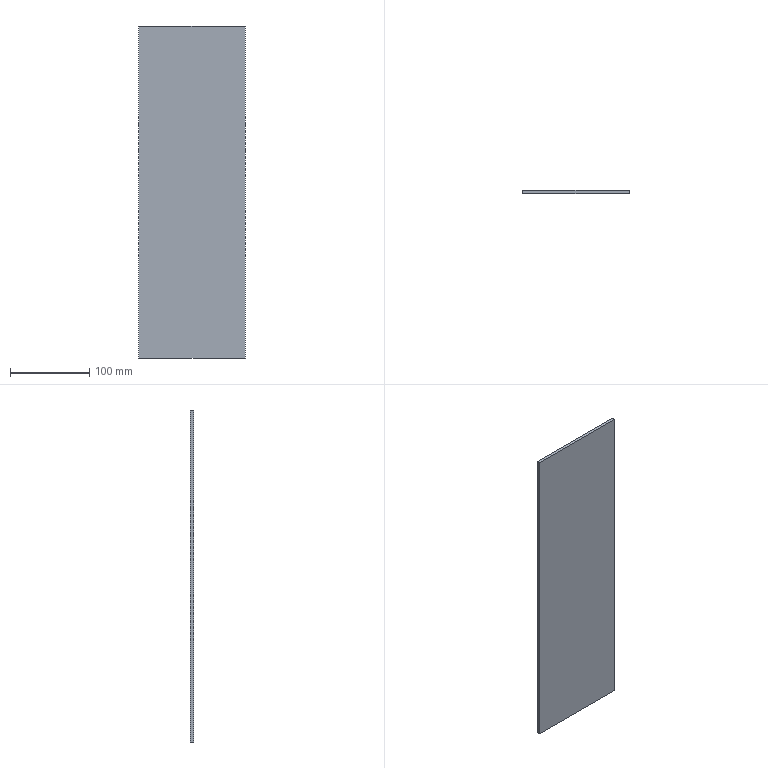Part | SolidWorks | features Extrusion 1, ICE 1 | 1 solid | 6 faces | box 135 x 4 x 420 mm | volume 226800 mm3 | plane 6
STEP:
#1=CARTESIAN_POINT('',(67.5,0.,210.));
#2=VERTEX_POINT('',#1);
#3=CARTESIAN_POINT('',(67.5,0.,-210.));
#4=VERTEX_POINT('',#3);
#5=CARTESIAN_POINT('',(67.5,0.,-210.));
#6=DIRECTION('',(0.,0.,-1.));
#7=VECTOR('',#6,1000.);
#8=LINE('',#5,#7);
#9=EDGE_CURVE('',#2,#4,#8,.T.);
#10=ORIENTED_EDGE('',*,*,#9,.T.);
#11=CARTESIAN_POINT('',(67.5,4.,-210.));
#12=VERTEX_POINT('',#11);
#13=CARTESIAN_POINT('',(67.5,4.,-210.));
#14=DIRECTION('',(0.,-1.,0.));
#15=VECTOR('',#14,1000.);
#16=LINE('',#13,#15);
#17=EDGE_CURVE('',#12,#4,#16,.T.);
#18=ORIENTED_EDGE('',*,*,#17,.F.);
#19=CARTESIAN_POINT('',(67.5,4.,210.));
#20=VERTEX_POINT('',#19);
#21=CARTESIAN_POINT('',(67.5,4.,-210.));
#22=DIRECTION('',(0.,0.,-1.));
#23=VECTOR('',#22,1000.);
#24=LINE('',#21,#23);
#25=EDGE_CURVE('',#20,#12,#24,.T.);
#26=ORIENTED_EDGE('',*,*,#25,.F.);
#27=CARTESIAN_POINT('',(67.5,4.,210.));
#28=DIRECTION('',(0.,-1.,0.));
#29=VECTOR('',#28,1000.);
#30=LINE('',#27,#29);
#31=EDGE_CURVE('',#20,#2,#30,.T.);
#32=ORIENTED_EDGE('',*,*,#31,.T.);
#33=EDGE_LOOP('',(#10,#18,#26,#32));
#34=FACE_OUTER_BOUND('',#33,.T.);
#35=CARTESIAN_POINT('',(67.5,4.,-210.));
#36=DIRECTION('',(-1.,0.,0.));
#37=DIRECTION('',(0.,0.,1.));
#38=AXIS2_PLACEMENT_3D('',#35,#36,#37);
#39=PLANE('',#38);
#40=ADVANCED_FACE('',(#34),#39,.F.);
#41=CARTESIAN_POINT('',(-67.5,0.,-210.));
#42=VERTEX_POINT('',#41);
#43=CARTESIAN_POINT('',(-67.5,0.,-210.));
#44=DIRECTION('',(-1.,0.,0.));
#45=VECTOR('',#44,1000.);
#46=LINE('',#43,#45);
#47=EDGE_CURVE('',#4,#42,#46,.T.);
#48=ORIENTED_EDGE('',*,*,#47,.T.);
#49=CARTESIAN_POINT('',(-67.5,4.,-210.));
#50=VERTEX_POINT('',#49);
#51=CARTESIAN_POINT('',(-67.5,4.,-210.));
#52=DIRECTION('',(0.,-1.,0.));
#53=VECTOR('',#52,1000.);
#54=LINE('',#51,#53);
#55=EDGE_CURVE('',#50,#42,#54,.T.);
#56=ORIENTED_EDGE('',*,*,#55,.F.);
#57=CARTESIAN_POINT('',(-67.5,4.,-210.));
#58=DIRECTION('',(-1.,0.,0.));
#59=VECTOR('',#58,1000.);
#60=LINE('',#57,#59);
#61=EDGE_CURVE('',#12,#50,#60,.T.);
#62=ORIENTED_EDGE('',*,*,#61,.F.);
#63=ORIENTED_EDGE('',*,*,#17,.T.);
#64=EDGE_LOOP('',(#48,#56,#62,#63));
#65=FACE_OUTER_BOUND('',#64,.T.);
#66=CARTESIAN_POINT('',(-67.5,4.,-210.));
#67=DIRECTION('',(0.,0.,1.));
#68=DIRECTION('',(1.,0.,0.));
#69=AXIS2_PLACEMENT_3D('',#66,#67,#68);
#70=PLANE('',#69);
#71=ADVANCED_FACE('',(#65),#70,.F.);
#72=CARTESIAN_POINT('',(-67.5,0.,210.));
#73=VERTEX_POINT('',#72);
#74=CARTESIAN_POINT('',(-67.5,0.,-210.));
#75=DIRECTION('',(0.,0.,1.));
#76=VECTOR('',#75,1000.);
#77=LINE('',#74,#76);
#78=EDGE_CURVE('',#42,#73,#77,.T.);
#79=ORIENTED_EDGE('',*,*,#78,.T.);
#80=CARTESIAN_POINT('',(-67.5,4.,210.));
#81=VERTEX_POINT('',#80);
#82=CARTESIAN_POINT('',(-67.5,4.,210.));
#83=DIRECTION('',(0.,-1.,0.));
#84=VECTOR('',#83,1000.);
#85=LINE('',#82,#84);
#86=EDGE_CURVE('',#81,#73,#85,.T.);
#87=ORIENTED_EDGE('',*,*,#86,.F.);
#88=CARTESIAN_POINT('',(-67.5,4.,-210.));
#89=DIRECTION('',(0.,0.,1.));
#90=VECTOR('',#89,1000.);
#91=LINE('',#88,#90);
#92=EDGE_CURVE('',#50,#81,#91,.T.);
#93=ORIENTED_EDGE('',*,*,#92,.F.);
#94=ORIENTED_EDGE('',*,*,#55,.T.);
#95=EDGE_LOOP('',(#79,#87,#93,#94));
#96=FACE_OUTER_BOUND('',#95,.T.);
#97=CARTESIAN_POINT('',(-67.5,4.,-210.));
#98=DIRECTION('',(1.,0.,0.));
#99=DIRECTION('',(0.,0.,-1.));
#100=AXIS2_PLACEMENT_3D('',#97,#98,#99);
#101=PLANE('',#100);
#102=ADVANCED_FACE('',(#96),#101,.F.);
#103=CARTESIAN_POINT('',(-67.5,0.,210.));
#104=DIRECTION('',(1.,0.,0.));
#105=VECTOR('',#104,1000.);
#106=LINE('',#103,#105);
#107=EDGE_CURVE('',#73,#2,#106,.T.);
#108=ORIENTED_EDGE('',*,*,#107,.T.);
#109=ORIENTED_EDGE('',*,*,#31,.F.);
#110=CARTESIAN_POINT('',(-67.5,4.,210.));
#111=DIRECTION('',(1.,0.,0.));
#112=VECTOR('',#111,1000.);
#113=LINE('',#110,#112);
#114=EDGE_CURVE('',#81,#20,#113,.T.);
#115=ORIENTED_EDGE('',*,*,#114,.F.);
#116=ORIENTED_EDGE('',*,*,#86,.T.);
#117=EDGE_LOOP('',(#108,#109,#115,#116));
#118=FACE_OUTER_BOUND('',#117,.T.);
#119=CARTESIAN_POINT('',(-67.5,4.,210.));
#120=DIRECTION('',(0.,0.,-1.));
#121=DIRECTION('',(-1.,0.,0.));
#122=AXIS2_PLACEMENT_3D('',#119,#120,#121);
#123=PLANE('',#122);
#124=ADVANCED_FACE('',(#118),#123,.F.);
#125=ORIENTED_EDGE('',*,*,#25,.T.);
#126=ORIENTED_EDGE('',*,*,#61,.T.);
#127=ORIENTED_EDGE('',*,*,#92,.T.);
#128=ORIENTED_EDGE('',*,*,#114,.T.);
#129=EDGE_LOOP('',(#125,#126,#127,#128));
#130=FACE_OUTER_BOUND('',#129,.T.);
#131=CARTESIAN_POINT('',(0.,4.,0.));
#132=DIRECTION('',(0.,1.,0.));
#133=DIRECTION('',(0.,0.,1.));
#134=AXIS2_PLACEMENT_3D('',#131,#132,#133);
#135=PLANE('',#134);
#136=ADVANCED_FACE('',(#130),#135,.T.);
#137=ORIENTED_EDGE('',*,*,#9,.F.);
#138=ORIENTED_EDGE('',*,*,#107,.F.);
#139=ORIENTED_EDGE('',*,*,#78,.F.);
#140=ORIENTED_EDGE('',*,*,#47,.F.);
#141=EDGE_LOOP('',(#137,#138,#139,#140));
#142=FACE_OUTER_BOUND('',#141,.T.);
#143=CARTESIAN_POINT('',(0.,0.,0.));
#144=DIRECTION('',(0.,1.,0.));
#145=DIRECTION('',(0.,0.,1.));
#146=AXIS2_PLACEMENT_3D('',#143,#144,#145);
#147=PLANE('',#146);
#148=ADVANCED_FACE('',(#142),#147,.F.);
#149=CLOSED_SHELL('',(#40,#71,#102,#124,#136,#148));
#150=MANIFOLD_SOLID_BREP('',#149);
#151=CARTESIAN_POINT('',(0.,0.,0.));
#152=DIRECTION('',(0.,0.,1.));
#153=DIRECTION('',(1.,0.,0.));
#154=AXIS2_PLACEMENT_3D('',#151,#152,#153);
#155=(LENGTH_UNIT()NAMED_UNIT(*)SI_UNIT(.MILLI.,.METRE.));
#156=UNCERTAINTY_MEASURE_WITH_UNIT(LENGTH_MEASURE(0.00001),#155,'','');
#157=(NAMED_UNIT(*)PLANE_ANGLE_UNIT()SI_UNIT($,.RADIAN.));
#158=(NAMED_UNIT(*)SI_UNIT($,.STERADIAN.)SOLID_ANGLE_UNIT());
#159=(GEOMETRIC_REPRESENTATION_CONTEXT(3)GLOBAL_UNCERTAINTY_ASSIGNED_CONTEXT((#156))GLOBAL_UNIT_ASSIGNED_CONTEXT((#155,#157,#158))REPRESENTATION_CONTEXT('',''));
#160=ADVANCED_BREP_SHAPE_REPRESENTATION('',(#150,#154),#159);